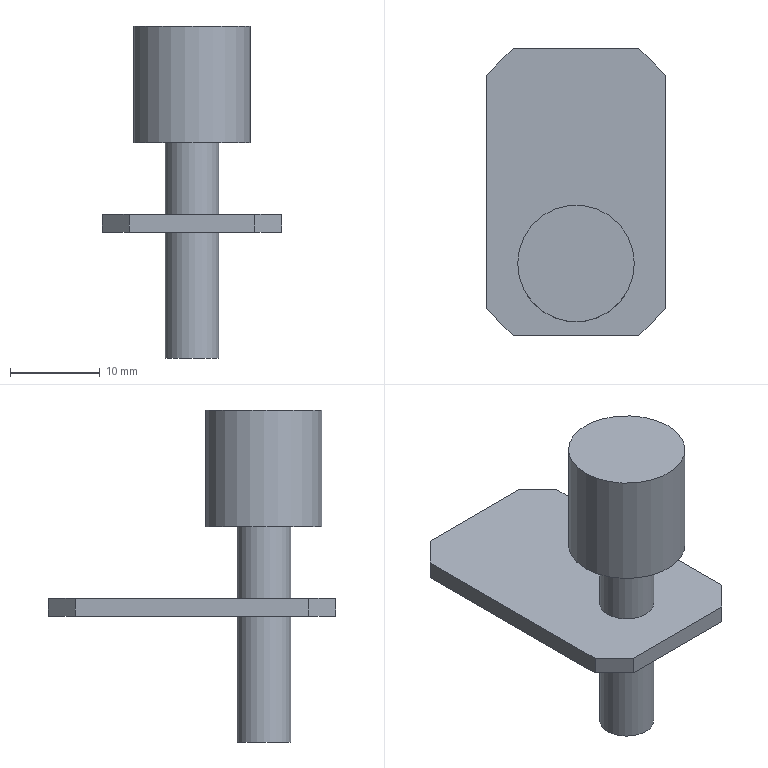Part | NX | 1 solid | 16 faces | box 20 x 32 x 37 mm | volume 3592 mm3 | plane 13 | cylinder 3 | commonest cylinder face diameters 6 x2 13 x1
STEP:
#1=CARTESIAN_POINT('',(3.,8.,-16.));
#2=VERTEX_POINT('',#1);
#3=CARTESIAN_POINT('',(0.,8.,-16.));
#4=DIRECTION('',(0.,0.,1.));
#5=DIRECTION('',(1.,0.,0.));
#6=AXIS2_PLACEMENT_3D('',#3,#4,#5);
#7=CIRCLE('',#6,3.);
#8=EDGE_CURVE('',#2,#2,#7,.T.);
#9=ORIENTED_EDGE('',*,*,#8,.T.);
#10=EDGE_LOOP('',(#9));
#11=FACE_BOUND('',#10,.T.);
#12=CARTESIAN_POINT('',(3.,8.,-2.));
#13=VERTEX_POINT('',#12);
#14=CARTESIAN_POINT('',(0.,8.,-2.));
#15=DIRECTION('',(0.,0.,1.));
#16=DIRECTION('',(1.,0.,0.));
#17=AXIS2_PLACEMENT_3D('',#14,#15,#16);
#18=CIRCLE('',#17,3.);
#19=EDGE_CURVE('',#13,#13,#18,.F.);
#20=ORIENTED_EDGE('',*,*,#19,.T.);
#21=EDGE_LOOP('',(#20));
#22=FACE_BOUND('',#21,.T.);
#23=CARTESIAN_POINT('',(0.,8.,8.));
#24=DIRECTION('',(0.,0.,-1.));
#25=DIRECTION('',(-1.,0.,0.));
#26=AXIS2_PLACEMENT_3D('',#23,#24,#25);
#27=CYLINDRICAL_SURFACE('',#26,3.);
#28=ADVANCED_FACE('',(#11,#22),#27,.T.);
#29=ORIENTED_EDGE('',*,*,#8,.F.);
#30=EDGE_LOOP('',(#29));
#31=FACE_BOUND('',#30,.T.);
#32=CARTESIAN_POINT('',(0.,8.,-16.));
#33=DIRECTION('',(0.,0.,1.));
#34=DIRECTION('',(1.,0.,0.));
#35=AXIS2_PLACEMENT_3D('',#32,#33,#34);
#36=PLANE('',#35);
#37=ADVANCED_FACE('',(#31),#36,.F.);
#38=CARTESIAN_POINT('',(10.,3.,-2.));
#39=VERTEX_POINT('',#38);
#40=CARTESIAN_POINT('',(10.,29.,-2.));
#41=VERTEX_POINT('',#40);
#42=CARTESIAN_POINT('',(10.,0.,-2.));
#43=DIRECTION('',(0.,1.,0.));
#44=VECTOR('',#43,1000.);
#45=LINE('',#42,#44);
#46=EDGE_CURVE('',#39,#41,#45,.T.);
#47=ORIENTED_EDGE('',*,*,#46,.F.);
#48=CARTESIAN_POINT('',(7.,0.,-2.));
#49=VERTEX_POINT('',#48);
#50=CARTESIAN_POINT('',(7.,0.,-2.));
#51=DIRECTION('',(-0.7071,-0.7071,0.));
#52=VECTOR('',#51,1000.);
#53=LINE('',#50,#52);
#54=EDGE_CURVE('',#39,#49,#53,.T.);
#55=ORIENTED_EDGE('',*,*,#54,.T.);
#56=CARTESIAN_POINT('',(-7.,0.,-2.));
#57=VERTEX_POINT('',#56);
#58=CARTESIAN_POINT('',(10.,0.,-2.));
#59=DIRECTION('',(-1.,0.,0.));
#60=VECTOR('',#59,1000.);
#61=LINE('',#58,#60);
#62=EDGE_CURVE('',#49,#57,#61,.T.);
#63=ORIENTED_EDGE('',*,*,#62,.T.);
#64=CARTESIAN_POINT('',(-10.,3.,-2.));
#65=VERTEX_POINT('',#64);
#66=CARTESIAN_POINT('',(-10.,3.,-2.));
#67=DIRECTION('',(0.7071,-0.7071,0.));
#68=VECTOR('',#67,1000.);
#69=LINE('',#66,#68);
#70=EDGE_CURVE('',#57,#65,#69,.F.);
#71=ORIENTED_EDGE('',*,*,#70,.T.);
#72=CARTESIAN_POINT('',(-10.,29.,-2.));
#73=VERTEX_POINT('',#72);
#74=CARTESIAN_POINT('',(-10.,0.,-2.));
#75=DIRECTION('',(0.,1.,0.));
#76=VECTOR('',#75,1000.);
#77=LINE('',#74,#76);
#78=EDGE_CURVE('',#65,#73,#77,.T.);
#79=ORIENTED_EDGE('',*,*,#78,.T.);
#80=CARTESIAN_POINT('',(-7.,32.,-2.));
#81=VERTEX_POINT('',#80);
#82=CARTESIAN_POINT('',(-10.,29.,-2.));
#83=DIRECTION('',(-0.7071,-0.7071,0.));
#84=VECTOR('',#83,1000.);
#85=LINE('',#82,#84);
#86=EDGE_CURVE('',#73,#81,#85,.F.);
#87=ORIENTED_EDGE('',*,*,#86,.T.);
#88=CARTESIAN_POINT('',(7.,32.,-2.));
#89=VERTEX_POINT('',#88);
#90=CARTESIAN_POINT('',(10.,32.,-2.));
#91=DIRECTION('',(-1.,0.,0.));
#92=VECTOR('',#91,1000.);
#93=LINE('',#90,#92);
#94=EDGE_CURVE('',#89,#81,#93,.T.);
#95=ORIENTED_EDGE('',*,*,#94,.F.);
#96=CARTESIAN_POINT('',(7.,32.,-2.));
#97=DIRECTION('',(0.7071,-0.7071,0.));
#98=VECTOR('',#97,1000.);
#99=LINE('',#96,#98);
#100=EDGE_CURVE('',#89,#41,#99,.T.);
#101=ORIENTED_EDGE('',*,*,#100,.T.);
#102=EDGE_LOOP('',(#47,#55,#63,#71,#79,#87,#95,#101));
#103=FACE_BOUND('',#102,.T.);
#104=ORIENTED_EDGE('',*,*,#19,.F.);
#105=EDGE_LOOP('',(#104));
#106=FACE_BOUND('',#105,.T.);
#107=CARTESIAN_POINT('',(10.,0.,-2.));
#108=DIRECTION('',(0.,0.,1.));
#109=DIRECTION('',(1.,0.,0.));
#110=AXIS2_PLACEMENT_3D('',#107,#108,#109);
#111=PLANE('',#110);
#112=ADVANCED_FACE('',(#103,#106),#111,.F.);
#113=CARTESIAN_POINT('',(7.,0.,0.));
#114=VERTEX_POINT('',#113);
#115=CARTESIAN_POINT('',(-7.,0.,0.));
#116=VERTEX_POINT('',#115);
#117=CARTESIAN_POINT('',(10.,0.,0.));
#118=DIRECTION('',(-1.,0.,0.));
#119=VECTOR('',#118,1000.);
#120=LINE('',#117,#119);
#121=EDGE_CURVE('',#114,#116,#120,.T.);
#122=ORIENTED_EDGE('',*,*,#121,.F.);
#123=CARTESIAN_POINT('',(10.,3.,0.));
#124=VERTEX_POINT('',#123);
#125=CARTESIAN_POINT('',(8.5,1.5,0.));
#126=DIRECTION('',(0.7071,0.7071,0.));
#127=VECTOR('',#126,1000.);
#128=LINE('',#125,#127);
#129=EDGE_CURVE('',#114,#124,#128,.T.);
#130=ORIENTED_EDGE('',*,*,#129,.T.);
#131=CARTESIAN_POINT('',(10.,29.,0.));
#132=VERTEX_POINT('',#131);
#133=CARTESIAN_POINT('',(10.,0.,0.));
#134=DIRECTION('',(0.,1.,0.));
#135=VECTOR('',#134,1000.);
#136=LINE('',#133,#135);
#137=EDGE_CURVE('',#124,#132,#136,.T.);
#138=ORIENTED_EDGE('',*,*,#137,.T.);
#139=CARTESIAN_POINT('',(7.,32.,0.));
#140=VERTEX_POINT('',#139);
#141=CARTESIAN_POINT('',(24.5,14.5,0.));
#142=DIRECTION('',(-0.7071,0.7071,0.));
#143=VECTOR('',#142,1000.);
#144=LINE('',#141,#143);
#145=EDGE_CURVE('',#132,#140,#144,.T.);
#146=ORIENTED_EDGE('',*,*,#145,.T.);
#147=CARTESIAN_POINT('',(-7.,32.,0.));
#148=VERTEX_POINT('',#147);
#149=CARTESIAN_POINT('',(10.,32.,0.));
#150=DIRECTION('',(-1.,0.,0.));
#151=VECTOR('',#150,1000.);
#152=LINE('',#149,#151);
#153=EDGE_CURVE('',#140,#148,#152,.T.);
#154=ORIENTED_EDGE('',*,*,#153,.T.);
#155=CARTESIAN_POINT('',(-10.,29.,0.));
#156=VERTEX_POINT('',#155);
#157=CARTESIAN_POINT('',(-14.5,24.5,0.));
#158=DIRECTION('',(0.7071,0.7071,0.));
#159=VECTOR('',#158,1000.);
#160=LINE('',#157,#159);
#161=EDGE_CURVE('',#148,#156,#160,.F.);
#162=ORIENTED_EDGE('',*,*,#161,.T.);
#163=CARTESIAN_POINT('',(-10.,3.,0.));
#164=VERTEX_POINT('',#163);
#165=CARTESIAN_POINT('',(-10.,0.,0.));
#166=DIRECTION('',(0.,1.,0.));
#167=VECTOR('',#166,1000.);
#168=LINE('',#165,#167);
#169=EDGE_CURVE('',#164,#156,#168,.T.);
#170=ORIENTED_EDGE('',*,*,#169,.F.);
#171=CARTESIAN_POINT('',(1.5,-8.5,0.));
#172=DIRECTION('',(-0.7071,0.7071,0.));
#173=VECTOR('',#172,1000.);
#174=LINE('',#171,#173);
#175=EDGE_CURVE('',#164,#116,#174,.F.);
#176=ORIENTED_EDGE('',*,*,#175,.T.);
#177=EDGE_LOOP('',(#122,#130,#138,#146,#154,#162,#170,#176));
#178=FACE_BOUND('',#177,.T.);
#179=CARTESIAN_POINT('',(3.,8.,0.));
#180=VERTEX_POINT('',#179);
#181=CARTESIAN_POINT('',(0.,8.,0.));
#182=DIRECTION('',(0.,0.,1.));
#183=DIRECTION('',(1.,0.,0.));
#184=AXIS2_PLACEMENT_3D('',#181,#182,#183);
#185=CIRCLE('',#184,3.);
#186=EDGE_CURVE('',#180,#180,#185,.F.);
#187=ORIENTED_EDGE('',*,*,#186,.T.);
#188=EDGE_LOOP('',(#187));
#189=FACE_BOUND('',#188,.T.);
#190=CARTESIAN_POINT('',(10.,0.,0.));
#191=DIRECTION('',(0.,0.,1.));
#192=DIRECTION('',(1.,0.,0.));
#193=AXIS2_PLACEMENT_3D('',#190,#191,#192);
#194=PLANE('',#193);
#195=ADVANCED_FACE('',(#178,#189),#194,.T.);
#196=ORIENTED_EDGE('',*,*,#153,.F.);
#197=CARTESIAN_POINT('',(7.,32.,-2.));
#198=DIRECTION('',(0.,0.,-1.));
#199=VECTOR('',#198,1000.);
#200=LINE('',#197,#199);
#201=EDGE_CURVE('',#140,#89,#200,.T.);
#202=ORIENTED_EDGE('',*,*,#201,.T.);
#203=ORIENTED_EDGE('',*,*,#94,.T.);
#204=CARTESIAN_POINT('',(-7.,32.,0.));
#205=DIRECTION('',(0.,0.,1.));
#206=VECTOR('',#205,1000.);
#207=LINE('',#204,#206);
#208=EDGE_CURVE('',#81,#148,#207,.T.);
#209=ORIENTED_EDGE('',*,*,#208,.T.);
#210=EDGE_LOOP('',(#196,#202,#203,#209));
#211=FACE_BOUND('',#210,.T.);
#212=CARTESIAN_POINT('',(10.,32.,0.));
#213=DIRECTION('',(0.,1.,0.));
#214=DIRECTION('',(0.,0.,1.));
#215=AXIS2_PLACEMENT_3D('',#212,#213,#214);
#216=PLANE('',#215);
#217=ADVANCED_FACE('',(#211),#216,.T.);
#218=ORIENTED_EDGE('',*,*,#62,.F.);
#219=CARTESIAN_POINT('',(7.,0.,0.));
#220=DIRECTION('',(0.,0.,1.));
#221=VECTOR('',#220,1000.);
#222=LINE('',#219,#221);
#223=EDGE_CURVE('',#49,#114,#222,.T.);
#224=ORIENTED_EDGE('',*,*,#223,.T.);
#225=ORIENTED_EDGE('',*,*,#121,.T.);
#226=CARTESIAN_POINT('',(-7.,0.,-2.));
#227=DIRECTION('',(0.,0.,-1.));
#228=VECTOR('',#227,1000.);
#229=LINE('',#226,#228);
#230=EDGE_CURVE('',#116,#57,#229,.T.);
#231=ORIENTED_EDGE('',*,*,#230,.T.);
#232=EDGE_LOOP('',(#218,#224,#225,#231));
#233=FACE_BOUND('',#232,.T.);
#234=CARTESIAN_POINT('',(10.,0.,-2.));
#235=DIRECTION('',(0.,-1.,0.));
#236=DIRECTION('',(0.,0.,-1.));
#237=AXIS2_PLACEMENT_3D('',#234,#235,#236);
#238=PLANE('',#237);
#239=ADVANCED_FACE('',(#233),#238,.T.);
#240=ORIENTED_EDGE('',*,*,#137,.F.);
#241=CARTESIAN_POINT('',(10.,3.,-2.));
#242=DIRECTION('',(0.,0.,-1.));
#243=VECTOR('',#242,1000.);
#244=LINE('',#241,#243);
#245=EDGE_CURVE('',#124,#39,#244,.T.);
#246=ORIENTED_EDGE('',*,*,#245,.T.);
#247=ORIENTED_EDGE('',*,*,#46,.T.);
#248=CARTESIAN_POINT('',(10.,29.,0.));
#249=DIRECTION('',(0.,0.,1.));
#250=VECTOR('',#249,1000.);
#251=LINE('',#248,#250);
#252=EDGE_CURVE('',#41,#132,#251,.T.);
#253=ORIENTED_EDGE('',*,*,#252,.T.);
#254=EDGE_LOOP('',(#240,#246,#247,#253));
#255=FACE_BOUND('',#254,.T.);
#256=CARTESIAN_POINT('',(10.,0.,0.));
#257=DIRECTION('',(-1.,0.,0.));
#258=DIRECTION('',(0.,0.,1.));
#259=AXIS2_PLACEMENT_3D('',#256,#257,#258);
#260=PLANE('',#259);
#261=ADVANCED_FACE('',(#255),#260,.F.);
#262=ORIENTED_EDGE('',*,*,#169,.T.);
#263=CARTESIAN_POINT('',(-10.,29.,0.));
#264=DIRECTION('',(0.,0.,-1.));
#265=VECTOR('',#264,1000.);
#266=LINE('',#263,#265);
#267=EDGE_CURVE('',#156,#73,#266,.T.);
#268=ORIENTED_EDGE('',*,*,#267,.T.);
#269=ORIENTED_EDGE('',*,*,#78,.F.);
#270=CARTESIAN_POINT('',(-10.,3.,0.));
#271=DIRECTION('',(0.,0.,1.));
#272=VECTOR('',#271,1000.);
#273=LINE('',#270,#272);
#274=EDGE_CURVE('',#65,#164,#273,.T.);
#275=ORIENTED_EDGE('',*,*,#274,.T.);
#276=EDGE_LOOP('',(#262,#268,#269,#275));
#277=FACE_BOUND('',#276,.T.);
#278=CARTESIAN_POINT('',(-10.,0.,0.));
#279=DIRECTION('',(-1.,0.,0.));
#280=DIRECTION('',(0.,0.,1.));
#281=AXIS2_PLACEMENT_3D('',#278,#279,#280);
#282=PLANE('',#281);
#283=ADVANCED_FACE('',(#277),#282,.T.);
#284=ORIENTED_EDGE('',*,*,#54,.F.);
#285=ORIENTED_EDGE('',*,*,#245,.F.);
#286=ORIENTED_EDGE('',*,*,#129,.F.);
#287=ORIENTED_EDGE('',*,*,#223,.F.);
#288=EDGE_LOOP('',(#284,#285,#286,#287));
#289=FACE_BOUND('',#288,.T.);
#290=CARTESIAN_POINT('',(7.,0.,-2.));
#291=DIRECTION('',(0.7071,-0.7071,0.));
#292=DIRECTION('',(0.,0.,-1.));
#293=AXIS2_PLACEMENT_3D('',#290,#291,#292);
#294=PLANE('',#293);
#295=ADVANCED_FACE('',(#289),#294,.T.);
#296=ORIENTED_EDGE('',*,*,#145,.F.);
#297=ORIENTED_EDGE('',*,*,#252,.F.);
#298=ORIENTED_EDGE('',*,*,#100,.F.);
#299=ORIENTED_EDGE('',*,*,#201,.F.);
#300=EDGE_LOOP('',(#296,#297,#298,#299));
#301=FACE_BOUND('',#300,.T.);
#302=CARTESIAN_POINT('',(7.,32.,0.));
#303=DIRECTION('',(0.7071,0.7071,0.));
#304=DIRECTION('',(0.,0.,1.));
#305=AXIS2_PLACEMENT_3D('',#302,#303,#304);
#306=PLANE('',#305);
#307=ADVANCED_FACE('',(#301),#306,.T.);
#308=ORIENTED_EDGE('',*,*,#161,.F.);
#309=ORIENTED_EDGE('',*,*,#208,.F.);
#310=ORIENTED_EDGE('',*,*,#86,.F.);
#311=ORIENTED_EDGE('',*,*,#267,.F.);
#312=EDGE_LOOP('',(#308,#309,#310,#311));
#313=FACE_BOUND('',#312,.T.);
#314=CARTESIAN_POINT('',(-10.,29.,0.));
#315=DIRECTION('',(0.7071,-0.7071,0.));
#316=DIRECTION('',(0.,0.,-1.));
#317=AXIS2_PLACEMENT_3D('',#314,#315,#316);
#318=PLANE('',#317);
#319=ADVANCED_FACE('',(#313),#318,.F.);
#320=ORIENTED_EDGE('',*,*,#70,.F.);
#321=ORIENTED_EDGE('',*,*,#230,.F.);
#322=ORIENTED_EDGE('',*,*,#175,.F.);
#323=ORIENTED_EDGE('',*,*,#274,.F.);
#324=EDGE_LOOP('',(#320,#321,#322,#323));
#325=FACE_BOUND('',#324,.T.);
#326=CARTESIAN_POINT('',(-10.,3.,0.));
#327=DIRECTION('',(0.7071,0.7071,0.));
#328=DIRECTION('',(0.,0.,1.));
#329=AXIS2_PLACEMENT_3D('',#326,#327,#328);
#330=PLANE('',#329);
#331=ADVANCED_FACE('',(#325),#330,.F.);
#332=ORIENTED_EDGE('',*,*,#186,.F.);
#333=EDGE_LOOP('',(#332));
#334=FACE_BOUND('',#333,.T.);
#335=CARTESIAN_POINT('',(3.,8.,8.));
#336=VERTEX_POINT('',#335);
#337=CARTESIAN_POINT('',(0.,8.,8.));
#338=DIRECTION('',(0.,0.,1.));
#339=DIRECTION('',(1.,0.,0.));
#340=AXIS2_PLACEMENT_3D('',#337,#338,#339);
#341=CIRCLE('',#340,3.);
#342=EDGE_CURVE('',#336,#336,#341,.T.);
#343=ORIENTED_EDGE('',*,*,#342,.F.);
#344=EDGE_LOOP('',(#343));
#345=FACE_BOUND('',#344,.T.);
#346=CARTESIAN_POINT('',(0.,8.,8.));
#347=DIRECTION('',(0.,0.,-1.));
#348=DIRECTION('',(-1.,0.,0.));
#349=AXIS2_PLACEMENT_3D('',#346,#347,#348);
#350=CYLINDRICAL_SURFACE('',#349,3.);
#351=ADVANCED_FACE('',(#334,#345),#350,.T.);
#352=CARTESIAN_POINT('',(6.5,8.,8.));
#353=VERTEX_POINT('',#352);
#354=CARTESIAN_POINT('',(0.,8.,8.));
#355=DIRECTION('',(0.,0.,1.));
#356=DIRECTION('',(1.,0.,0.));
#357=AXIS2_PLACEMENT_3D('',#354,#355,#356);
#358=CIRCLE('',#357,6.5);
#359=EDGE_CURVE('',#353,#353,#358,.T.);
#360=ORIENTED_EDGE('',*,*,#359,.F.);
#361=EDGE_LOOP('',(#360));
#362=FACE_BOUND('',#361,.T.);
#363=ORIENTED_EDGE('',*,*,#342,.T.);
#364=EDGE_LOOP('',(#363));
#365=FACE_BOUND('',#364,.T.);
#366=CARTESIAN_POINT('',(0.,8.,8.));
#367=DIRECTION('',(0.,0.,1.));
#368=DIRECTION('',(1.,0.,0.));
#369=AXIS2_PLACEMENT_3D('',#366,#367,#368);
#370=PLANE('',#369);
#371=ADVANCED_FACE('',(#362,#365),#370,.F.);
#372=CARTESIAN_POINT('',(6.5,8.,21.));
#373=VERTEX_POINT('',#372);
#374=CARTESIAN_POINT('',(0.,8.,21.));
#375=DIRECTION('',(0.,0.,1.));
#376=DIRECTION('',(1.,0.,0.));
#377=AXIS2_PLACEMENT_3D('',#374,#375,#376);
#378=CIRCLE('',#377,6.5);
#379=EDGE_CURVE('',#373,#373,#378,.T.);
#380=ORIENTED_EDGE('',*,*,#379,.F.);
#381=EDGE_LOOP('',(#380));
#382=FACE_BOUND('',#381,.T.);
#383=ORIENTED_EDGE('',*,*,#359,.T.);
#384=EDGE_LOOP('',(#383));
#385=FACE_BOUND('',#384,.T.);
#386=CARTESIAN_POINT('',(0.,8.,21.));
#387=DIRECTION('',(0.,0.,-1.));
#388=DIRECTION('',(-1.,0.,0.));
#389=AXIS2_PLACEMENT_3D('',#386,#387,#388);
#390=CYLINDRICAL_SURFACE('',#389,6.5);
#391=ADVANCED_FACE('',(#382,#385),#390,.T.);
#392=ORIENTED_EDGE('',*,*,#379,.T.);
#393=EDGE_LOOP('',(#392));
#394=FACE_BOUND('',#393,.T.);
#395=CARTESIAN_POINT('',(0.,8.,21.));
#396=DIRECTION('',(0.,0.,1.));
#397=DIRECTION('',(1.,0.,0.));
#398=AXIS2_PLACEMENT_3D('',#395,#396,#397);
#399=PLANE('',#398);
#400=ADVANCED_FACE('',(#394),#399,.T.);
#401=CLOSED_SHELL('',(#28,#37,#112,#195,#217,#239,#261,#283,#295,#307,#319,#331,#351,#371,#391,#400));
#402=MANIFOLD_SOLID_BREP('',#401);
#403=(LENGTH_UNIT()NAMED_UNIT(*)SI_UNIT(.MILLI.,.METRE.));
#404=UNCERTAINTY_MEASURE_WITH_UNIT(LENGTH_MEASURE(0.00001),#403,'','');
#405=(NAMED_UNIT(*)PLANE_ANGLE_UNIT()SI_UNIT($,.RADIAN.));
#406=(NAMED_UNIT(*)SI_UNIT($,.STERADIAN.)SOLID_ANGLE_UNIT());
#407=(GEOMETRIC_REPRESENTATION_CONTEXT(3)GLOBAL_UNCERTAINTY_ASSIGNED_CONTEXT((#404))GLOBAL_UNIT_ASSIGNED_CONTEXT((#403,#405,#406))REPRESENTATION_CONTEXT('',''));
#408=ADVANCED_BREP_SHAPE_REPRESENTATION('',(#402),#407);